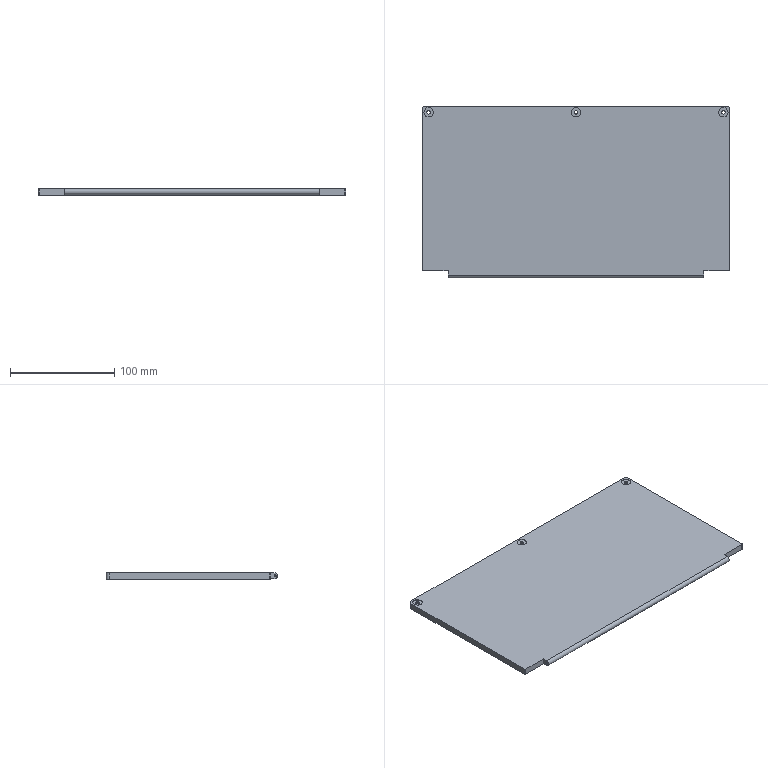CAM job | Mastercam | 3-axis milling, drilling
Tools:
tool_number,name,type,diameter_mm,corner_radius_mm,flutes,flute_length_mm,overall_length_mm,shoulder_length_mm,holder_diameter_mm,length_offset,diameter_offset,default_rpm,default_feed_mm_min,default_plunge_mm_min,coolant
1,4 Bull Nose Mill,bull end mill,4,1,4,25,100,25,50,1,1,10000,3000,600,COOL_OFF
3,3 Flat End Mill,end mill,3,0,4,25,75,25,50,3,3,7000,2000,600,COOL_OFF
5,4 Chamfer Mill,chamfer mill,4,0,4,25,75,30,50,5,5,3000,300,600,COOL_OFF
6,6 Flat End Mill,end mill,6,0,4,25,75,25,50,6,6,7000,3000,600,COOL_OFF
8,8 Flat End Mill,end mill,8,0,4,25,75,25,50,8,8,7000,3000,600,COOL_OFF
9,10 Flat End Mill,end mill,10,0,4,25,75,25,50,9,9,7000,3000,600,COOL_OFF
10,10 Flat End Mill,end mill,10,0,4,25,75,25,50,10,10,7000,1000,600,COOL_OFF
Operations:
seq,operation,operation_type,tool_number,tool_name,tool_diameter_mm,spindle_rpm,feed_mm_min,plunge_mm_min,retract_mm_min,cycle_time_s,wcs,posted,nc_file
1,Contour (Ramp) - [WCS: Plane] - [Tplane: Plane],Contour,9,10 Flat End Mill,10,7000,3000,600,1200,21.982,Plane,yes,.nc
2,Contour (Ramp) - [WCS: Plane] - [Tplane: Plane],Contour,9,10 Flat End Mill,10,7000,3000,600,1200,244.311,Plane,yes,.nc
3,Contour (2D) - [WCS: Plane] - [Tplane: Plane],Contour,10,10 Flat End Mill,10,7000,1000,600,1200,58.103,Plane,yes,.nc
4,Surface Finish Flowline - [WCS: Plane] - [Tplane: Plane],MultiSurfaceFinishFlowline,1,4 Bull Nose Mill,4,10000,3000,600,1200,282.467,Plane,yes,.nc
5,Helix Bore - [WCS: Plane] - [Tplane: Plane],HelixBore,6,6 Flat End Mill,6,7000,3000,600,1200,12.294,Plane,yes,.nc
6,Drill/Counterbore - [WCS: Plane] - [Tplane: Plane],Drill,5,4 Chamfer Mill,4,3000,300,600,1200,2.456,Plane,yes,.nc
7,Contour (2D chamfer) - [WCS: Plane] - [Tplane: Plane],Contour,5,4 Chamfer Mill,4,7000,1000,600,1200,6.915,Plane,yes,.nc
8,Contour (2D chamfer) - [WCS: Plane] - [Tplane: Plane],Contour,5,4 Chamfer Mill,4,7000,1000,600,1200,55.738,Plane,yes,.nc
9,2D High Speed (2D Area Mill) - [WCS: Plane-1] - [Tplane: Plane-1],HighSpeed2D,6,6 Flat End Mill,6,7000,3000,600,1200,2446.468,Plane-1,yes,.nc
10,Contour (2D) - [WCS: Plane-1] - [Tplane: Plane-1],Contour,6,6 Flat End Mill,6,7000,1000,600,1200,51.867,Plane-1,yes,.nc
11,Surface Finish Flowline - [WCS: Plane-1] - [Tplane: Plane-1],MultiSurfaceFinishFlowline,1,4 Bull Nose Mill,4,10000,3000,600,1200,282.471,Plane-1,yes,.nc
12,Contour (Ramp) - [WCS: Plane-1] - [Tplane: Plane-1],Contour,6,6 Flat End Mill,6,7000,3000,600,1200,5.995,Plane-1,yes,.nc
13,Contour (2D) - [WCS: Plane-1] - [Tplane: Plane-1],Contour,6,6 Flat End Mill,6,7000,1000,600,1200,16.781,Plane-1,yes,.nc
14,Helix Bore - [WCS: Plane-1] - [Tplane: Plane-1],HelixBore,3,3 Flat End Mill,3,7000,2000,600,1200,24.717,Plane-1,yes,.nc
15,Contour (2D chamfer) - [WCS: Plane-1] - [Tplane: Plane-1],Contour,5,4 Chamfer Mill,4,7000,1000,600,1200,94.397,Plane-1,yes,.nc
16,Contour (2D chamfer) - [WCS: Plane-1] - [Tplane: Plane-1],Contour,5,4 Chamfer Mill,4,7000,1000,600,1200,18.31,Plane-1,yes,.nc
17,Contour (Ramp) - [WCS: Plane-2] - [Tplane: Plane-2],Contour,8,8 Flat End Mill,8,7000,3000,600,1200,24.764,Plane-2,yes,.nc
18,Contour (2D) - [WCS: Plane-2] - [Tplane: Plane-2],Contour,8,8 Flat End Mill,8,7000,1000,600,1200,8.069,Plane-2,yes,.nc
19,Drill/Counterbore - [WCS: Plane-2] - [Tplane: Plane-2],Drill,5,4 Chamfer Mill,4,3000,300,600,1200,0.819,Plane-2,yes,.nc
20,Contour (Ramp) - [WCS: Plane-3] - [Tplane: Plane-3],Contour,8,8 Flat End Mill,8,7000,3000,600,1200,25.164,Plane-3,yes,.nc
21,Contour (2D) - [WCS: Plane-3] - [Tplane: Plane-3],Contour,8,8 Flat End Mill,8,7000,1000,600,1200,8.144,Plane-3,yes,.nc
22,Drill/Counterbore - [WCS: Plane-3] - [Tplane: Plane-3],Drill,5,4 Chamfer Mill,4,3000,300,600,1200,0.819,Plane-3,yes,.nc